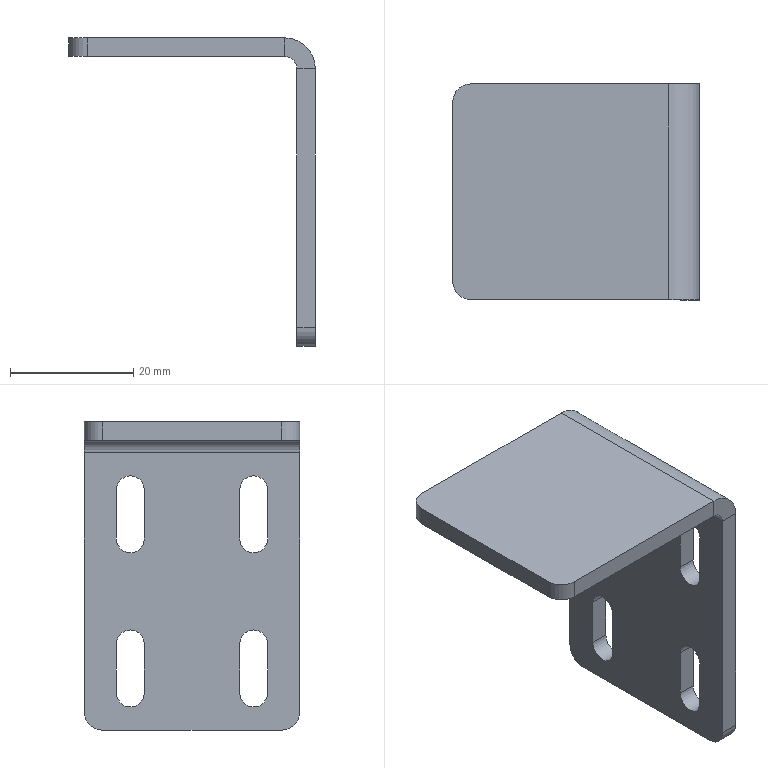Part | SolidWorks | features EdgeFlange 3, RefAxis 3, Fillet 2, ICE 2, FlatPattern 1, SMBaseFlange 1, SheetMetal 1 | 1 solid | 38 faces | box 40 x 35 x 50 mm | volume 8331 mm3 | plane 20 | cylinder 18 | commonest cylinder face diameters 4.5 x12 6 x4 4 x1 10 x1
STEP:
#1=CARTESIAN_POINT('',(55.,-7.75,-36.));
#2=VERTEX_POINT('',#1);
#3=CARTESIAN_POINT('',(55.,-10.,-33.75));
#4=VERTEX_POINT('',#3);
#5=CARTESIAN_POINT('',(55.,-10.,-36.));
#6=DIRECTION('',(1.,0.,0.));
#7=DIRECTION('',(0.,0.,-1.));
#8=AXIS2_PLACEMENT_3D('',#5,#6,#7);
#9=CIRCLE('',#8,2.25);
#10=EDGE_CURVE('',#2,#4,#9,.T.);
#11=ORIENTED_EDGE('',*,*,#10,.T.);
#12=CARTESIAN_POINT('',(52.,-10.,-33.75));
#13=VERTEX_POINT('',#12);
#14=CARTESIAN_POINT('',(62.,-10.,-33.75));
#15=DIRECTION('',(-1.,0.,0.));
#16=VECTOR('',#15,1000.);
#17=LINE('',#14,#16);
#18=EDGE_CURVE('',#4,#13,#17,.T.);
#19=ORIENTED_EDGE('',*,*,#18,.T.);
#20=CARTESIAN_POINT('',(52.,-7.75,-36.));
#21=VERTEX_POINT('',#20);
#22=CARTESIAN_POINT('',(52.,-10.,-36.));
#23=DIRECTION('',(-1.,0.,0.));
#24=DIRECTION('',(0.,0.,-1.));
#25=AXIS2_PLACEMENT_3D('',#22,#23,#24);
#26=CIRCLE('',#25,2.25);
#27=EDGE_CURVE('',#13,#21,#26,.T.);
#28=ORIENTED_EDGE('',*,*,#27,.T.);
#29=CARTESIAN_POINT('',(62.,-7.75,-36.));
#30=DIRECTION('',(-1.,0.,0.));
#31=VECTOR('',#30,1000.);
#32=LINE('',#29,#31);
#33=EDGE_CURVE('',#2,#21,#32,.T.);
#34=ORIENTED_EDGE('',*,*,#33,.F.);
#35=EDGE_LOOP('',(#11,#19,#28,#34));
#36=FACE_OUTER_BOUND('',#35,.T.);
#37=CARTESIAN_POINT('',(62.,-10.,-36.));
#38=DIRECTION('',(-1.,0.,0.));
#39=DIRECTION('',(0.,0.,1.));
#40=AXIS2_PLACEMENT_3D('',#37,#38,#39);
#41=CYLINDRICAL_SURFACE('',#40,2.25);
#42=ADVANCED_FACE('',(#36),#41,.F.);
#43=CARTESIAN_POINT('',(55.,-7.75,-11.));
#44=VERTEX_POINT('',#43);
#45=CARTESIAN_POINT('',(55.,-10.,-8.75));
#46=VERTEX_POINT('',#45);
#47=CARTESIAN_POINT('',(55.,-10.,-11.));
#48=DIRECTION('',(1.,0.,0.));
#49=DIRECTION('',(0.,0.,-1.));
#50=AXIS2_PLACEMENT_3D('',#47,#48,#49);
#51=CIRCLE('',#50,2.25);
#52=EDGE_CURVE('',#44,#46,#51,.T.);
#53=ORIENTED_EDGE('',*,*,#52,.T.);
#54=CARTESIAN_POINT('',(52.,-10.,-8.75));
#55=VERTEX_POINT('',#54);
#56=CARTESIAN_POINT('',(62.,-10.,-8.75));
#57=DIRECTION('',(-1.,0.,0.));
#58=VECTOR('',#57,1000.);
#59=LINE('',#56,#58);
#60=EDGE_CURVE('',#46,#55,#59,.T.);
#61=ORIENTED_EDGE('',*,*,#60,.T.);
#62=CARTESIAN_POINT('',(52.,-7.75,-11.));
#63=VERTEX_POINT('',#62);
#64=CARTESIAN_POINT('',(52.,-10.,-11.));
#65=DIRECTION('',(-1.,0.,0.));
#66=DIRECTION('',(0.,0.,1.));
#67=AXIS2_PLACEMENT_3D('',#64,#65,#66);
#68=CIRCLE('',#67,2.25);
#69=EDGE_CURVE('',#55,#63,#68,.T.);
#70=ORIENTED_EDGE('',*,*,#69,.T.);
#71=CARTESIAN_POINT('',(62.,-7.75,-11.));
#72=DIRECTION('',(-1.,0.,0.));
#73=VECTOR('',#72,1000.);
#74=LINE('',#71,#73);
#75=EDGE_CURVE('',#44,#63,#74,.T.);
#76=ORIENTED_EDGE('',*,*,#75,.F.);
#77=EDGE_LOOP('',(#53,#61,#70,#76));
#78=FACE_OUTER_BOUND('',#77,.T.);
#79=CARTESIAN_POINT('',(62.,-10.,-11.));
#80=DIRECTION('',(-1.,0.,0.));
#81=DIRECTION('',(0.,0.,1.));
#82=AXIS2_PLACEMENT_3D('',#79,#80,#81);
#83=CYLINDRICAL_SURFACE('',#82,2.25);
#84=ADVANCED_FACE('',(#78),#83,.F.);
#85=CARTESIAN_POINT('',(55.,12.25,-11.));
#86=VERTEX_POINT('',#85);
#87=CARTESIAN_POINT('',(55.,10.,-8.75));
#88=VERTEX_POINT('',#87);
#89=CARTESIAN_POINT('',(55.,10.,-11.));
#90=DIRECTION('',(1.,0.,0.));
#91=DIRECTION('',(0.,0.,-1.));
#92=AXIS2_PLACEMENT_3D('',#89,#90,#91);
#93=CIRCLE('',#92,2.25);
#94=EDGE_CURVE('',#86,#88,#93,.T.);
#95=ORIENTED_EDGE('',*,*,#94,.T.);
#96=CARTESIAN_POINT('',(52.,10.,-8.75));
#97=VERTEX_POINT('',#96);
#98=CARTESIAN_POINT('',(62.,10.,-8.75));
#99=DIRECTION('',(-1.,0.,0.));
#100=VECTOR('',#99,1000.);
#101=LINE('',#98,#100);
#102=EDGE_CURVE('',#88,#97,#101,.T.);
#103=ORIENTED_EDGE('',*,*,#102,.T.);
#104=CARTESIAN_POINT('',(52.,12.25,-11.));
#105=VERTEX_POINT('',#104);
#106=CARTESIAN_POINT('',(52.,10.,-11.));
#107=DIRECTION('',(-1.,0.,0.));
#108=DIRECTION('',(0.,0.,-1.));
#109=AXIS2_PLACEMENT_3D('',#106,#107,#108);
#110=CIRCLE('',#109,2.25);
#111=EDGE_CURVE('',#97,#105,#110,.T.);
#112=ORIENTED_EDGE('',*,*,#111,.T.);
#113=CARTESIAN_POINT('',(62.,12.25,-11.));
#114=DIRECTION('',(-1.,0.,0.));
#115=VECTOR('',#114,1000.);
#116=LINE('',#113,#115);
#117=EDGE_CURVE('',#86,#105,#116,.T.);
#118=ORIENTED_EDGE('',*,*,#117,.F.);
#119=EDGE_LOOP('',(#95,#103,#112,#118));
#120=FACE_OUTER_BOUND('',#119,.T.);
#121=CARTESIAN_POINT('',(62.,10.,-11.));
#122=DIRECTION('',(-1.,0.,0.));
#123=DIRECTION('',(0.,0.,1.));
#124=AXIS2_PLACEMENT_3D('',#121,#122,#123);
#125=CYLINDRICAL_SURFACE('',#124,2.25);
#126=ADVANCED_FACE('',(#120),#125,.F.);
#127=CARTESIAN_POINT('',(55.,12.25,-36.));
#128=VERTEX_POINT('',#127);
#129=CARTESIAN_POINT('',(55.,10.,-33.75));
#130=VERTEX_POINT('',#129);
#131=CARTESIAN_POINT('',(55.,10.,-36.));
#132=DIRECTION('',(1.,0.,0.));
#133=DIRECTION('',(0.,0.,-1.));
#134=AXIS2_PLACEMENT_3D('',#131,#132,#133);
#135=CIRCLE('',#134,2.25);
#136=EDGE_CURVE('',#128,#130,#135,.T.);
#137=ORIENTED_EDGE('',*,*,#136,.T.);
#138=CARTESIAN_POINT('',(52.,10.,-33.75));
#139=VERTEX_POINT('',#138);
#140=CARTESIAN_POINT('',(62.,10.,-33.75));
#141=DIRECTION('',(-1.,0.,0.));
#142=VECTOR('',#141,1000.);
#143=LINE('',#140,#142);
#144=EDGE_CURVE('',#130,#139,#143,.T.);
#145=ORIENTED_EDGE('',*,*,#144,.T.);
#146=CARTESIAN_POINT('',(52.,12.25,-36.));
#147=VERTEX_POINT('',#146);
#148=CARTESIAN_POINT('',(52.,10.,-36.));
#149=DIRECTION('',(-1.,0.,0.));
#150=DIRECTION('',(0.,0.,1.));
#151=AXIS2_PLACEMENT_3D('',#148,#149,#150);
#152=CIRCLE('',#151,2.25);
#153=EDGE_CURVE('',#139,#147,#152,.T.);
#154=ORIENTED_EDGE('',*,*,#153,.T.);
#155=CARTESIAN_POINT('',(62.,12.25,-36.));
#156=DIRECTION('',(-1.,0.,0.));
#157=VECTOR('',#156,1000.);
#158=LINE('',#155,#157);
#159=EDGE_CURVE('',#128,#147,#158,.T.);
#160=ORIENTED_EDGE('',*,*,#159,.F.);
#161=EDGE_LOOP('',(#137,#145,#154,#160));
#162=FACE_OUTER_BOUND('',#161,.T.);
#163=CARTESIAN_POINT('',(62.,10.,-36.));
#164=DIRECTION('',(-1.,0.,0.));
#165=DIRECTION('',(0.,0.,1.));
#166=AXIS2_PLACEMENT_3D('',#163,#164,#165);
#167=CYLINDRICAL_SURFACE('',#166,2.25);
#168=ADVANCED_FACE('',(#162),#167,.F.);
#169=CARTESIAN_POINT('',(18.,-17.5,0.));
#170=VERTEX_POINT('',#169);
#171=CARTESIAN_POINT('',(50.,-17.5,0.));
#172=VERTEX_POINT('',#171);
#173=CARTESIAN_POINT('',(-55.,-17.5,0.));
#174=DIRECTION('',(1.,0.,0.));
#175=VECTOR('',#174,1000.);
#176=LINE('',#173,#175);
#177=EDGE_CURVE('',#170,#172,#176,.T.);
#178=ORIENTED_EDGE('',*,*,#177,.F.);
#179=CARTESIAN_POINT('',(18.,-17.5,-3.));
#180=VERTEX_POINT('',#179);
#181=CARTESIAN_POINT('',(18.,-17.5,-3.));
#182=DIRECTION('',(0.,0.,-1.));
#183=VECTOR('',#182,1000.);
#184=LINE('',#181,#183);
#185=EDGE_CURVE('',#170,#180,#184,.T.);
#186=ORIENTED_EDGE('',*,*,#185,.T.);
#187=CARTESIAN_POINT('',(50.,-17.5,-3.));
#188=VERTEX_POINT('',#187);
#189=CARTESIAN_POINT('',(-55.,-17.5,-3.));
#190=DIRECTION('',(1.,0.,0.));
#191=VECTOR('',#190,1000.);
#192=LINE('',#189,#191);
#193=EDGE_CURVE('',#180,#188,#192,.T.);
#194=ORIENTED_EDGE('',*,*,#193,.T.);
#195=CARTESIAN_POINT('',(50.,-17.5,-3.));
#196=DIRECTION('',(0.,0.,1.));
#197=VECTOR('',#196,1000.);
#198=LINE('',#195,#197);
#199=EDGE_CURVE('',#188,#172,#198,.T.);
#200=ORIENTED_EDGE('',*,*,#199,.T.);
#201=EDGE_LOOP('',(#178,#186,#194,#200));
#202=FACE_OUTER_BOUND('',#201,.T.);
#203=CARTESIAN_POINT('',(-55.,-17.5,-3.));
#204=DIRECTION('',(0.,-1.,0.));
#205=DIRECTION('',(0.,0.,-1.));
#206=AXIS2_PLACEMENT_3D('',#203,#204,#205);
#207=PLANE('',#206);
#208=ADVANCED_FACE('',(#202),#207,.T.);
#209=ORIENTED_EDGE('',*,*,#193,.F.);
#210=CARTESIAN_POINT('',(15.,-14.5,-3.));
#211=VERTEX_POINT('',#210);
#212=CARTESIAN_POINT('',(18.,-14.5,-3.));
#213=DIRECTION('',(0.,0.,-1.));
#214=DIRECTION('',(-1.,0.,0.));
#215=AXIS2_PLACEMENT_3D('',#212,#213,#214);
#216=CIRCLE('',#215,3.);
#217=EDGE_CURVE('',#180,#211,#216,.T.);
#218=ORIENTED_EDGE('',*,*,#217,.T.);
#219=CARTESIAN_POINT('',(15.,14.5,-3.));
#220=VERTEX_POINT('',#219);
#221=CARTESIAN_POINT('',(15.,-17.5,-3.));
#222=DIRECTION('',(0.,1.,0.));
#223=VECTOR('',#222,1000.);
#224=LINE('',#221,#223);
#225=EDGE_CURVE('',#211,#220,#224,.T.);
#226=ORIENTED_EDGE('',*,*,#225,.T.);
#227=CARTESIAN_POINT('',(18.,17.5,-3.));
#228=VERTEX_POINT('',#227);
#229=CARTESIAN_POINT('',(18.,14.5,-3.));
#230=DIRECTION('',(0.,0.,-1.));
#231=DIRECTION('',(-1.,0.,0.));
#232=AXIS2_PLACEMENT_3D('',#229,#230,#231);
#233=CIRCLE('',#232,3.);
#234=EDGE_CURVE('',#220,#228,#233,.T.);
#235=ORIENTED_EDGE('',*,*,#234,.T.);
#236=CARTESIAN_POINT('',(50.,17.5,-3.));
#237=VERTEX_POINT('',#236);
#238=CARTESIAN_POINT('',(-55.,17.5,-3.));
#239=DIRECTION('',(-1.,0.,0.));
#240=VECTOR('',#239,1000.);
#241=LINE('',#238,#240);
#242=EDGE_CURVE('',#237,#228,#241,.T.);
#243=ORIENTED_EDGE('',*,*,#242,.F.);
#244=CARTESIAN_POINT('',(50.,-17.5,-3.));
#245=DIRECTION('',(0.,1.,0.));
#246=VECTOR('',#245,1000.);
#247=LINE('',#244,#246);
#248=EDGE_CURVE('',#188,#237,#247,.T.);
#249=ORIENTED_EDGE('',*,*,#248,.F.);
#250=EDGE_LOOP('',(#209,#218,#226,#235,#243,#249));
#251=FACE_OUTER_BOUND('',#250,.T.);
#252=CARTESIAN_POINT('',(0.,0.,-3.));
#253=DIRECTION('',(0.,0.,-1.));
#254=DIRECTION('',(-1.,0.,0.));
#255=AXIS2_PLACEMENT_3D('',#252,#253,#254);
#256=PLANE('',#255);
#257=ADVANCED_FACE('',(#251),#256,.T.);
#258=CARTESIAN_POINT('',(15.,14.5,0.));
#259=VERTEX_POINT('',#258);
#260=CARTESIAN_POINT('',(15.,-14.5,0.));
#261=VERTEX_POINT('',#260);
#262=CARTESIAN_POINT('',(15.,0.,0.));
#263=DIRECTION('',(0.,-1.,0.));
#264=VECTOR('',#263,1000.);
#265=LINE('',#262,#264);
#266=EDGE_CURVE('',#259,#261,#265,.T.);
#267=ORIENTED_EDGE('',*,*,#266,.T.);
#268=CARTESIAN_POINT('',(18.,-14.5,0.));
#269=DIRECTION('',(0.,0.,1.));
#270=DIRECTION('',(-1.,0.,0.));
#271=AXIS2_PLACEMENT_3D('',#268,#269,#270);
#272=CIRCLE('',#271,3.);
#273=EDGE_CURVE('',#261,#170,#272,.T.);
#274=ORIENTED_EDGE('',*,*,#273,.T.);
#275=ORIENTED_EDGE('',*,*,#177,.T.);
#276=CARTESIAN_POINT('',(50.,17.5,0.));
#277=VERTEX_POINT('',#276);
#278=CARTESIAN_POINT('',(50.,-17.5,0.));
#279=DIRECTION('',(0.,1.,0.));
#280=VECTOR('',#279,1000.);
#281=LINE('',#278,#280);
#282=EDGE_CURVE('',#172,#277,#281,.T.);
#283=ORIENTED_EDGE('',*,*,#282,.T.);
#284=CARTESIAN_POINT('',(18.,17.5,0.));
#285=VERTEX_POINT('',#284);
#286=CARTESIAN_POINT('',(-55.,17.5,0.));
#287=DIRECTION('',(-1.,0.,0.));
#288=VECTOR('',#287,1000.);
#289=LINE('',#286,#288);
#290=EDGE_CURVE('',#277,#285,#289,.T.);
#291=ORIENTED_EDGE('',*,*,#290,.T.);
#292=CARTESIAN_POINT('',(18.,14.5,0.));
#293=DIRECTION('',(0.,0.,1.));
#294=DIRECTION('',(-1.,0.,0.));
#295=AXIS2_PLACEMENT_3D('',#292,#293,#294);
#296=CIRCLE('',#295,3.);
#297=EDGE_CURVE('',#285,#259,#296,.T.);
#298=ORIENTED_EDGE('',*,*,#297,.T.);
#299=EDGE_LOOP('',(#267,#274,#275,#283,#291,#298));
#300=FACE_OUTER_BOUND('',#299,.T.);
#301=CARTESIAN_POINT('',(0.,0.,0.));
#302=DIRECTION('',(0.,0.,-1.));
#303=DIRECTION('',(-1.,0.,0.));
#304=AXIS2_PLACEMENT_3D('',#301,#302,#303);
#305=PLANE('',#304);
#306=ADVANCED_FACE('',(#300),#305,.F.);
#307=ORIENTED_EDGE('',*,*,#242,.T.);
#308=CARTESIAN_POINT('',(18.,17.5,0.));
#309=DIRECTION('',(0.,0.,1.));
#310=VECTOR('',#309,1000.);
#311=LINE('',#308,#310);
#312=EDGE_CURVE('',#228,#285,#311,.T.);
#313=ORIENTED_EDGE('',*,*,#312,.T.);
#314=ORIENTED_EDGE('',*,*,#290,.F.);
#315=CARTESIAN_POINT('',(50.,17.5,-3.));
#316=DIRECTION('',(0.,0.,1.));
#317=VECTOR('',#316,1000.);
#318=LINE('',#315,#317);
#319=EDGE_CURVE('',#237,#277,#318,.T.);
#320=ORIENTED_EDGE('',*,*,#319,.F.);
#321=EDGE_LOOP('',(#307,#313,#314,#320));
#322=FACE_OUTER_BOUND('',#321,.T.);
#323=CARTESIAN_POINT('',(-55.,17.5,-3.));
#324=DIRECTION('',(0.,1.,0.));
#325=DIRECTION('',(0.,0.,1.));
#326=AXIS2_PLACEMENT_3D('',#323,#324,#325);
#327=PLANE('',#326);
#328=ADVANCED_FACE('',(#322),#327,.T.);
#329=CARTESIAN_POINT('',(52.,17.5,-5.));
#330=VERTEX_POINT('',#329);
#331=CARTESIAN_POINT('',(55.,17.5,-5.));
#332=VERTEX_POINT('',#331);
#333=CARTESIAN_POINT('',(55.,17.5,-5.));
#334=DIRECTION('',(1.,0.,0.));
#335=VECTOR('',#334,1000.);
#336=LINE('',#333,#335);
#337=EDGE_CURVE('',#330,#332,#336,.T.);
#338=ORIENTED_EDGE('',*,*,#337,.F.);
#339=CARTESIAN_POINT('',(50.,17.5,-5.));
#340=DIRECTION('',(0.,1.,0.));
#341=DIRECTION('',(0.,0.,-1.));
#342=AXIS2_PLACEMENT_3D('',#339,#340,#341);
#343=CIRCLE('',#342,2.);
#344=EDGE_CURVE('',#237,#330,#343,.T.);
#345=ORIENTED_EDGE('',*,*,#344,.F.);
#346=ORIENTED_EDGE('',*,*,#319,.T.);
#347=CARTESIAN_POINT('',(50.,17.5,-5.));
#348=DIRECTION('',(0.,1.,0.));
#349=DIRECTION('',(0.,0.,-1.));
#350=AXIS2_PLACEMENT_3D('',#347,#348,#349);
#351=CIRCLE('',#350,5.);
#352=EDGE_CURVE('',#277,#332,#351,.T.);
#353=ORIENTED_EDGE('',*,*,#352,.T.);
#354=EDGE_LOOP('',(#338,#345,#346,#353));
#355=FACE_OUTER_BOUND('',#354,.T.);
#356=CARTESIAN_POINT('',(50.,17.5,-5.));
#357=DIRECTION('',(0.,1.,0.));
#358=DIRECTION('',(0.,0.,1.));
#359=AXIS2_PLACEMENT_3D('',#356,#357,#358);
#360=PLANE('',#359);
#361=ADVANCED_FACE('',(#355),#360,.T.);
#362=CARTESIAN_POINT('',(52.,-17.5,-5.));
#363=VERTEX_POINT('',#362);
#364=CARTESIAN_POINT('',(50.,-17.5,-5.));
#365=DIRECTION('',(0.,-1.,0.));
#366=DIRECTION('',(0.,0.,-1.));
#367=AXIS2_PLACEMENT_3D('',#364,#365,#366);
#368=CIRCLE('',#367,2.);
#369=EDGE_CURVE('',#363,#188,#368,.T.);
#370=ORIENTED_EDGE('',*,*,#369,.F.);
#371=CARTESIAN_POINT('',(55.,-17.5,-5.));
#372=VERTEX_POINT('',#371);
#373=CARTESIAN_POINT('',(52.,-17.5,-5.));
#374=DIRECTION('',(1.,0.,0.));
#375=VECTOR('',#374,1000.);
#376=LINE('',#373,#375);
#377=EDGE_CURVE('',#363,#372,#376,.T.);
#378=ORIENTED_EDGE('',*,*,#377,.T.);
#379=CARTESIAN_POINT('',(50.,-17.5,-5.));
#380=DIRECTION('',(0.,-1.,0.));
#381=DIRECTION('',(0.,0.,-1.));
#382=AXIS2_PLACEMENT_3D('',#379,#380,#381);
#383=CIRCLE('',#382,5.);
#384=EDGE_CURVE('',#372,#172,#383,.T.);
#385=ORIENTED_EDGE('',*,*,#384,.T.);
#386=ORIENTED_EDGE('',*,*,#199,.F.);
#387=EDGE_LOOP('',(#370,#378,#385,#386));
#388=FACE_OUTER_BOUND('',#387,.T.);
#389=CARTESIAN_POINT('',(50.,-17.5,-5.));
#390=DIRECTION('',(0.,1.,0.));
#391=DIRECTION('',(0.,0.,1.));
#392=AXIS2_PLACEMENT_3D('',#389,#390,#391);
#393=PLANE('',#392);
#394=ADVANCED_FACE('',(#388),#393,.F.);
#395=ORIENTED_EDGE('',*,*,#282,.F.);
#396=ORIENTED_EDGE('',*,*,#384,.F.);
#397=CARTESIAN_POINT('',(55.,0.,-5.));
#398=DIRECTION('',(0.,-1.,0.));
#399=VECTOR('',#398,1000.);
#400=LINE('',#397,#399);
#401=EDGE_CURVE('',#332,#372,#400,.T.);
#402=ORIENTED_EDGE('',*,*,#401,.F.);
#403=ORIENTED_EDGE('',*,*,#352,.F.);
#404=EDGE_LOOP('',(#395,#396,#402,#403));
#405=FACE_OUTER_BOUND('',#404,.T.);
#406=CARTESIAN_POINT('',(50.,-17.5,-5.));
#407=DIRECTION('',(0.,-1.,0.));
#408=DIRECTION('',(1.,0.,0.));
#409=AXIS2_PLACEMENT_3D('',#406,#407,#408);
#410=CYLINDRICAL_SURFACE('',#409,5.);
#411=ADVANCED_FACE('',(#405),#410,.T.);
#412=ORIENTED_EDGE('',*,*,#248,.T.);
#413=ORIENTED_EDGE('',*,*,#344,.T.);
#414=CARTESIAN_POINT('',(52.,17.5,-5.));
#415=DIRECTION('',(0.,-1.,0.));
#416=VECTOR('',#415,1000.);
#417=LINE('',#414,#416);
#418=EDGE_CURVE('',#330,#363,#417,.T.);
#419=ORIENTED_EDGE('',*,*,#418,.T.);
#420=ORIENTED_EDGE('',*,*,#369,.T.);
#421=EDGE_LOOP('',(#412,#413,#419,#420));
#422=FACE_OUTER_BOUND('',#421,.T.);
#423=CARTESIAN_POINT('',(50.,-17.5,-5.));
#424=DIRECTION('',(0.,-1.,0.));
#425=DIRECTION('',(1.,0.,0.));
#426=AXIS2_PLACEMENT_3D('',#423,#424,#425);
#427=CYLINDRICAL_SURFACE('',#426,2.);
#428=ADVANCED_FACE('',(#422),#427,.F.);
#429=CARTESIAN_POINT('',(52.,-17.5,-47.));
#430=VERTEX_POINT('',#429);
#431=CARTESIAN_POINT('',(52.,-17.5,0.));
#432=DIRECTION('',(0.,0.,1.));
#433=VECTOR('',#432,1000.);
#434=LINE('',#431,#433);
#435=EDGE_CURVE('',#430,#363,#434,.T.);
#436=ORIENTED_EDGE('',*,*,#435,.F.);
#437=CARTESIAN_POINT('',(55.,-17.5,-47.));
#438=VERTEX_POINT('',#437);
#439=CARTESIAN_POINT('',(55.,-17.5,-47.));
#440=DIRECTION('',(1.,0.,0.));
#441=VECTOR('',#440,1000.);
#442=LINE('',#439,#441);
#443=EDGE_CURVE('',#430,#438,#442,.T.);
#444=ORIENTED_EDGE('',*,*,#443,.T.);
#445=CARTESIAN_POINT('',(55.,-17.5,-3.));
#446=DIRECTION('',(0.,0.,1.));
#447=VECTOR('',#446,1000.);
#448=LINE('',#445,#447);
#449=EDGE_CURVE('',#438,#372,#448,.T.);
#450=ORIENTED_EDGE('',*,*,#449,.T.);
#451=ORIENTED_EDGE('',*,*,#377,.F.);
#452=EDGE_LOOP('',(#436,#444,#450,#451));
#453=FACE_OUTER_BOUND('',#452,.T.);
#454=CARTESIAN_POINT('',(55.,-17.5,-3.));
#455=DIRECTION('',(0.,-1.,0.));
#456=DIRECTION('',(0.,0.,-1.));
#457=AXIS2_PLACEMENT_3D('',#454,#455,#456);
#458=PLANE('',#457);
#459=ADVANCED_FACE('',(#453),#458,.T.);
#460=CARTESIAN_POINT('',(55.,17.5,-47.));
#461=VERTEX_POINT('',#460);
#462=CARTESIAN_POINT('',(55.,17.5,-50.));
#463=DIRECTION('',(0.,0.,-1.));
#464=VECTOR('',#463,1000.);
#465=LINE('',#462,#464);
#466=EDGE_CURVE('',#332,#461,#465,.T.);
#467=ORIENTED_EDGE('',*,*,#466,.T.);
#468=CARTESIAN_POINT('',(52.,17.5,-47.));
#469=VERTEX_POINT('',#468);
#470=CARTESIAN_POINT('',(55.,17.5,-47.));
#471=DIRECTION('',(-1.,0.,0.));
#472=VECTOR('',#471,1000.);
#473=LINE('',#470,#472);
#474=EDGE_CURVE('',#461,#469,#473,.T.);
#475=ORIENTED_EDGE('',*,*,#474,.T.);
#476=CARTESIAN_POINT('',(52.,17.5,0.));
#477=DIRECTION('',(0.,0.,-1.));
#478=VECTOR('',#477,1000.);
#479=LINE('',#476,#478);
#480=EDGE_CURVE('',#330,#469,#479,.T.);
#481=ORIENTED_EDGE('',*,*,#480,.F.);
#482=ORIENTED_EDGE('',*,*,#337,.T.);
#483=EDGE_LOOP('',(#467,#475,#481,#482));
#484=FACE_OUTER_BOUND('',#483,.T.);
#485=CARTESIAN_POINT('',(55.,17.5,-50.));
#486=DIRECTION('',(0.,1.,0.));
#487=DIRECTION('',(0.,0.,1.));
#488=AXIS2_PLACEMENT_3D('',#485,#486,#487);
#489=PLANE('',#488);
#490=ADVANCED_FACE('',(#484),#489,.T.);
#491=ORIENTED_EDGE('',*,*,#10,.F.);
#492=CARTESIAN_POINT('',(55.,-7.75,-44.));
#493=VERTEX_POINT('',#492);
#494=CARTESIAN_POINT('',(55.,-7.75,0.));
#495=DIRECTION('',(0.,0.,1.));
#496=VECTOR('',#495,1000.);
#497=LINE('',#494,#496);
#498=EDGE_CURVE('',#493,#2,#497,.T.);
#499=ORIENTED_EDGE('',*,*,#498,.F.);
#500=CARTESIAN_POINT('',(55.,-12.25,-44.));
#501=VERTEX_POINT('',#500);
#502=CARTESIAN_POINT('',(55.,-10.,-44.));
#503=DIRECTION('',(1.,0.,0.));
#504=DIRECTION('',(0.,0.,-1.));
#505=AXIS2_PLACEMENT_3D('',#502,#503,#504);
#506=CIRCLE('',#505,2.25);
#507=EDGE_CURVE('',#501,#493,#506,.T.);
#508=ORIENTED_EDGE('',*,*,#507,.F.);
#509=CARTESIAN_POINT('',(55.,-12.25,-36.));
#510=VERTEX_POINT('',#509);
#511=CARTESIAN_POINT('',(55.,-12.25,0.));
#512=DIRECTION('',(0.,0.,-1.));
#513=VECTOR('',#512,1000.);
#514=LINE('',#511,#513);
#515=EDGE_CURVE('',#510,#501,#514,.T.);
#516=ORIENTED_EDGE('',*,*,#515,.F.);
#517=CARTESIAN_POINT('',(55.,-10.,-36.));
#518=DIRECTION('',(1.,0.,0.));
#519=DIRECTION('',(0.,0.,-1.));
#520=AXIS2_PLACEMENT_3D('',#517,#518,#519);
#521=CIRCLE('',#520,2.25);
#522=EDGE_CURVE('',#4,#510,#521,.T.);
#523=ORIENTED_EDGE('',*,*,#522,.F.);
#524=EDGE_LOOP('',(#491,#499,#508,#516,#523));
#525=FACE_BOUND('',#524,.T.);
#526=CARTESIAN_POINT('',(55.,-12.25,-19.));
#527=VERTEX_POINT('',#526);
#528=CARTESIAN_POINT('',(55.,-7.75,-19.));
#529=VERTEX_POINT('',#528);
#530=CARTESIAN_POINT('',(55.,-10.,-19.));
#531=DIRECTION('',(1.,0.,0.));
#532=DIRECTION('',(0.,0.,-1.));
#533=AXIS2_PLACEMENT_3D('',#530,#531,#532);
#534=CIRCLE('',#533,2.25);
#535=EDGE_CURVE('',#527,#529,#534,.T.);
#536=ORIENTED_EDGE('',*,*,#535,.F.);
#537=CARTESIAN_POINT('',(55.,-12.25,-11.));
#538=VERTEX_POINT('',#537);
#539=CARTESIAN_POINT('',(55.,-12.25,0.));
#540=DIRECTION('',(0.,0.,-1.));
#541=VECTOR('',#540,1000.);
#542=LINE('',#539,#541);
#543=EDGE_CURVE('',#538,#527,#542,.T.);
#544=ORIENTED_EDGE('',*,*,#543,.F.);
#545=CARTESIAN_POINT('',(55.,-10.,-11.));
#546=DIRECTION('',(1.,0.,0.));
#547=DIRECTION('',(0.,0.,-1.));
#548=AXIS2_PLACEMENT_3D('',#545,#546,#547);
#549=CIRCLE('',#548,2.25);
#550=EDGE_CURVE('',#46,#538,#549,.T.);
#551=ORIENTED_EDGE('',*,*,#550,.F.);
#552=ORIENTED_EDGE('',*,*,#52,.F.);
#553=CARTESIAN_POINT('',(55.,-7.75,0.));
#554=DIRECTION('',(0.,0.,1.));
#555=VECTOR('',#554,1000.);
#556=LINE('',#553,#555);
#557=EDGE_CURVE('',#529,#44,#556,.T.);
#558=ORIENTED_EDGE('',*,*,#557,.F.);
#559=EDGE_LOOP('',(#536,#544,#551,#552,#558));
#560=FACE_BOUND('',#559,.T.);
#561=CARTESIAN_POINT('',(55.,7.75,-19.));
#562=VERTEX_POINT('',#561);
#563=CARTESIAN_POINT('',(55.,12.25,-19.));
#564=VERTEX_POINT('',#563);
#565=CARTESIAN_POINT('',(55.,10.,-19.));
#566=DIRECTION('',(1.,0.,0.));
#567=DIRECTION('',(0.,0.,-1.));
#568=AXIS2_PLACEMENT_3D('',#565,#566,#567);
#569=CIRCLE('',#568,2.25);
#570=EDGE_CURVE('',#562,#564,#569,.T.);
#571=ORIENTED_EDGE('',*,*,#570,.F.);
#572=CARTESIAN_POINT('',(55.,7.75,-11.));
#573=VERTEX_POINT('',#572);
#574=CARTESIAN_POINT('',(55.,7.75,0.));
#575=DIRECTION('',(0.,0.,-1.));
#576=VECTOR('',#575,1000.);
#577=LINE('',#574,#576);
#578=EDGE_CURVE('',#573,#562,#577,.T.);
#579=ORIENTED_EDGE('',*,*,#578,.F.);
#580=CARTESIAN_POINT('',(55.,10.,-11.));
#581=DIRECTION('',(1.,0.,0.));
#582=DIRECTION('',(0.,0.,-1.));
#583=AXIS2_PLACEMENT_3D('',#580,#581,#582);
#584=CIRCLE('',#583,2.25);
#585=EDGE_CURVE('',#88,#573,#584,.T.);
#586=ORIENTED_EDGE('',*,*,#585,.F.);
#587=ORIENTED_EDGE('',*,*,#94,.F.);
#588=CARTESIAN_POINT('',(55.,12.25,0.));
#589=DIRECTION('',(0.,0.,1.));
#590=VECTOR('',#589,1000.);
#591=LINE('',#588,#590);
#592=EDGE_CURVE('',#564,#86,#591,.T.);
#593=ORIENTED_EDGE('',*,*,#592,.F.);
#594=EDGE_LOOP('',(#571,#579,#586,#587,#593));
#595=FACE_BOUND('',#594,.T.);
#596=ORIENTED_EDGE('',*,*,#136,.F.);
#597=CARTESIAN_POINT('',(55.,12.25,-44.));
#598=VERTEX_POINT('',#597);
#599=CARTESIAN_POINT('',(55.,12.25,0.));
#600=DIRECTION('',(0.,0.,1.));
#601=VECTOR('',#600,1000.);
#602=LINE('',#599,#601);
#603=EDGE_CURVE('',#598,#128,#602,.T.);
#604=ORIENTED_EDGE('',*,*,#603,.F.);
#605=CARTESIAN_POINT('',(55.,7.75,-44.));
#606=VERTEX_POINT('',#605);
#607=CARTESIAN_POINT('',(55.,10.,-44.));
#608=DIRECTION('',(1.,0.,0.));
#609=DIRECTION('',(0.,0.,-1.));
#610=AXIS2_PLACEMENT_3D('',#607,#608,#609);
#611=CIRCLE('',#610,2.25);
#612=EDGE_CURVE('',#606,#598,#611,.T.);
#613=ORIENTED_EDGE('',*,*,#612,.F.);
#614=CARTESIAN_POINT('',(55.,7.75,-36.));
#615=VERTEX_POINT('',#614);
#616=CARTESIAN_POINT('',(55.,7.75,0.));
#617=DIRECTION('',(0.,0.,-1.));
#618=VECTOR('',#617,1000.);
#619=LINE('',#616,#618);
#620=EDGE_CURVE('',#615,#606,#619,.T.);
#621=ORIENTED_EDGE('',*,*,#620,.F.);
#622=CARTESIAN_POINT('',(55.,10.,-36.));
#623=DIRECTION('',(1.,0.,0.));
#624=DIRECTION('',(0.,0.,-1.));
#625=AXIS2_PLACEMENT_3D('',#622,#623,#624);
#626=CIRCLE('',#625,2.25);
#627=EDGE_CURVE('',#130,#615,#626,.T.);
#628=ORIENTED_EDGE('',*,*,#627,.F.);
#629=EDGE_LOOP('',(#596,#604,#613,#621,#628));
#630=FACE_BOUND('',#629,.T.);
#631=ORIENTED_EDGE('',*,*,#449,.F.);
#632=CARTESIAN_POINT('',(55.,-14.5,-50.));
#633=VERTEX_POINT('',#632);
#634=CARTESIAN_POINT('',(55.,-14.5,-47.));
#635=DIRECTION('',(1.,0.,0.));
#636=DIRECTION('',(0.,0.,-1.));
#637=AXIS2_PLACEMENT_3D('',#634,#635,#636);
#638=CIRCLE('',#637,3.);
#639=EDGE_CURVE('',#438,#633,#638,.T.);
#640=ORIENTED_EDGE('',*,*,#639,.T.);
#641=CARTESIAN_POINT('',(55.,14.5,-50.));
#642=VERTEX_POINT('',#641);
#643=CARTESIAN_POINT('',(55.,-17.5,-50.));
#644=DIRECTION('',(0.,-1.,0.));
#645=VECTOR('',#644,1000.);
#646=LINE('',#643,#645);
#647=EDGE_CURVE('',#642,#633,#646,.T.);
#648=ORIENTED_EDGE('',*,*,#647,.F.);
#649=CARTESIAN_POINT('',(55.,14.5,-47.));
#650=DIRECTION('',(1.,0.,0.));
#651=DIRECTION('',(0.,0.,-1.));
#652=AXIS2_PLACEMENT_3D('',#649,#650,#651);
#653=CIRCLE('',#652,3.);
#654=EDGE_CURVE('',#642,#461,#653,.T.);
#655=ORIENTED_EDGE('',*,*,#654,.T.);
#656=ORIENTED_EDGE('',*,*,#466,.F.);
#657=ORIENTED_EDGE('',*,*,#401,.T.);
#658=EDGE_LOOP('',(#631,#640,#648,#655,#656,#657));
#659=FACE_OUTER_BOUND('',#658,.T.);
#660=CARTESIAN_POINT('',(55.,0.,0.));
#661=DIRECTION('',(1.,0.,0.));
#662=DIRECTION('',(0.,0.,-1.));
#663=AXIS2_PLACEMENT_3D('',#660,#661,#662);
#664=PLANE('',#663);
#665=ADVANCED_FACE('',(#525,#560,#595,#630,#659),#664,.T.);
#666=CARTESIAN_POINT('',(52.,-7.75,-44.));
#667=VERTEX_POINT('',#666);
#668=CARTESIAN_POINT('',(52.,-7.75,-36.));
#669=DIRECTION('',(0.,0.,-1.));
#670=VECTOR('',#669,1000.);
#671=LINE('',#668,#670);
#672=EDGE_CURVE('',#21,#667,#671,.T.);
#673=ORIENTED_EDGE('',*,*,#672,.F.);
#674=ORIENTED_EDGE('',*,*,#27,.F.);
#675=CARTESIAN_POINT('',(52.,-12.25,-36.));
#676=VERTEX_POINT('',#675);
#677=CARTESIAN_POINT('',(52.,-10.,-36.));
#678=DIRECTION('',(-1.,0.,0.));
#679=DIRECTION('',(0.,0.,-1.));
#680=AXIS2_PLACEMENT_3D('',#677,#678,#679);
#681=CIRCLE('',#680,2.25);
#682=EDGE_CURVE('',#676,#13,#681,.T.);
#683=ORIENTED_EDGE('',*,*,#682,.F.);
#684=CARTESIAN_POINT('',(52.,-12.25,-44.));
#685=VERTEX_POINT('',#684);
#686=CARTESIAN_POINT('',(52.,-12.25,-36.));
#687=DIRECTION('',(0.,0.,1.));
#688=VECTOR('',#687,1000.);
#689=LINE('',#686,#688);
#690=EDGE_CURVE('',#685,#676,#689,.T.);
#691=ORIENTED_EDGE('',*,*,#690,.F.);
#692=CARTESIAN_POINT('',(52.,-10.,-44.));
#693=DIRECTION('',(-1.,0.,0.));
#694=DIRECTION('',(0.,0.,-1.));
#695=AXIS2_PLACEMENT_3D('',#692,#693,#694);
#696=CIRCLE('',#695,2.25);
#697=EDGE_CURVE('',#667,#685,#696,.T.);
#698=ORIENTED_EDGE('',*,*,#697,.F.);
#699=EDGE_LOOP('',(#673,#674,#683,#691,#698));
#700=FACE_BOUND('',#699,.T.);
#701=CARTESIAN_POINT('',(52.,-12.25,-19.));
#702=VERTEX_POINT('',#701);
#703=CARTESIAN_POINT('',(52.,-12.25,-11.));
#704=VERTEX_POINT('',#703);
#705=CARTESIAN_POINT('',(52.,-12.25,-19.));
#706=DIRECTION('',(0.,0.,1.));
#707=VECTOR('',#706,1000.);
#708=LINE('',#705,#707);
#709=EDGE_CURVE('',#702,#704,#708,.T.);
#710=ORIENTED_EDGE('',*,*,#709,.F.);
#711=CARTESIAN_POINT('',(52.,-7.75,-19.));
#712=VERTEX_POINT('',#711);
#713=CARTESIAN_POINT('',(52.,-10.,-19.));
#714=DIRECTION('',(-1.,0.,0.));
#715=DIRECTION('',(0.,0.,1.));
#716=AXIS2_PLACEMENT_3D('',#713,#714,#715);
#717=CIRCLE('',#716,2.25);
#718=EDGE_CURVE('',#712,#702,#717,.T.);
#719=ORIENTED_EDGE('',*,*,#718,.F.);
#720=CARTESIAN_POINT('',(52.,-7.75,-19.));
#721=DIRECTION('',(0.,0.,-1.));
#722=VECTOR('',#721,1000.);
#723=LINE('',#720,#722);
#724=EDGE_CURVE('',#63,#712,#723,.T.);
#725=ORIENTED_EDGE('',*,*,#724,.F.);
#726=ORIENTED_EDGE('',*,*,#69,.F.);
#727=CARTESIAN_POINT('',(52.,-10.,-11.));
#728=DIRECTION('',(-1.,0.,0.));
#729=DIRECTION('',(0.,0.,1.));
#730=AXIS2_PLACEMENT_3D('',#727,#728,#729);
#731=CIRCLE('',#730,2.25);
#732=EDGE_CURVE('',#704,#55,#731,.T.);
#733=ORIENTED_EDGE('',*,*,#732,.F.);
#734=EDGE_LOOP('',(#710,#719,#725,#726,#733));
#735=FACE_BOUND('',#734,.T.);
#736=CARTESIAN_POINT('',(52.,7.75,-19.));
#737=VERTEX_POINT('',#736);
#738=CARTESIAN_POINT('',(52.,7.75,-11.));
#739=VERTEX_POINT('',#738);
#740=CARTESIAN_POINT('',(52.,7.75,-19.));
#741=DIRECTION('',(0.,0.,1.));
#742=VECTOR('',#741,1000.);
#743=LINE('',#740,#742);
#744=EDGE_CURVE('',#737,#739,#743,.T.);
#745=ORIENTED_EDGE('',*,*,#744,.F.);
#746=CARTESIAN_POINT('',(52.,12.25,-19.));
#747=VERTEX_POINT('',#746);
#748=CARTESIAN_POINT('',(52.,10.,-19.));
#749=DIRECTION('',(-1.,0.,0.));
#750=DIRECTION('',(0.,0.,-1.));
#751=AXIS2_PLACEMENT_3D('',#748,#749,#750);
#752=CIRCLE('',#751,2.25);
#753=EDGE_CURVE('',#747,#737,#752,.T.);
#754=ORIENTED_EDGE('',*,*,#753,.F.);
#755=CARTESIAN_POINT('',(52.,12.25,-19.));
#756=DIRECTION('',(0.,0.,-1.));
#757=VECTOR('',#756,1000.);
#758=LINE('',#755,#757);
#759=EDGE_CURVE('',#105,#747,#758,.T.);
#760=ORIENTED_EDGE('',*,*,#759,.F.);
#761=ORIENTED_EDGE('',*,*,#111,.F.);
#762=CARTESIAN_POINT('',(52.,10.,-11.));
#763=DIRECTION('',(-1.,0.,0.));
#764=DIRECTION('',(0.,0.,-1.));
#765=AXIS2_PLACEMENT_3D('',#762,#763,#764);
#766=CIRCLE('',#765,2.25);
#767=EDGE_CURVE('',#739,#97,#766,.T.);
#768=ORIENTED_EDGE('',*,*,#767,.F.);
#769=EDGE_LOOP('',(#745,#754,#760,#761,#768));
#770=FACE_BOUND('',#769,.T.);
#771=CARTESIAN_POINT('',(52.,12.25,-44.));
#772=VERTEX_POINT('',#771);
#773=CARTESIAN_POINT('',(52.,12.25,-36.));
#774=DIRECTION('',(0.,0.,-1.));
#775=VECTOR('',#774,1000.);
#776=LINE('',#773,#775);
#777=EDGE_CURVE('',#147,#772,#776,.T.);
#778=ORIENTED_EDGE('',*,*,#777,.F.);
#779=ORIENTED_EDGE('',*,*,#153,.F.);
#780=CARTESIAN_POINT('',(52.,7.75,-36.));
#781=VERTEX_POINT('',#780);
#782=CARTESIAN_POINT('',(52.,10.,-36.));
#783=DIRECTION('',(-1.,0.,0.));
#784=DIRECTION('',(0.,0.,1.));
#785=AXIS2_PLACEMENT_3D('',#782,#783,#784);
#786=CIRCLE('',#785,2.25);
#787=EDGE_CURVE('',#781,#139,#786,.T.);
#788=ORIENTED_EDGE('',*,*,#787,.F.);
#789=CARTESIAN_POINT('',(52.,7.75,-44.));
#790=VERTEX_POINT('',#789);
#791=CARTESIAN_POINT('',(52.,7.75,-36.));
#792=DIRECTION('',(0.,0.,1.));
#793=VECTOR('',#792,1000.);
#794=LINE('',#791,#793);
#795=EDGE_CURVE('',#790,#781,#794,.T.);
#796=ORIENTED_EDGE('',*,*,#795,.F.);
#797=CARTESIAN_POINT('',(52.,10.,-44.));
#798=DIRECTION('',(-1.,0.,0.));
#799=DIRECTION('',(0.,0.,1.));
#800=AXIS2_PLACEMENT_3D('',#797,#798,#799);
#801=CIRCLE('',#800,2.25);
#802=EDGE_CURVE('',#772,#790,#801,.T.);
#803=ORIENTED_EDGE('',*,*,#802,.F.);
#804=EDGE_LOOP('',(#778,#779,#788,#796,#803));
#805=FACE_BOUND('',#804,.T.);
#806=CARTESIAN_POINT('',(52.,14.5,-50.));
#807=VERTEX_POINT('',#806);
#808=CARTESIAN_POINT('',(52.,-14.5,-50.));
#809=VERTEX_POINT('',#808);
#810=CARTESIAN_POINT('',(52.,0.,-50.));
#811=DIRECTION('',(0.,-1.,0.));
#812=VECTOR('',#811,1000.);
#813=LINE('',#810,#812);
#814=EDGE_CURVE('',#807,#809,#813,.T.);
#815=ORIENTED_EDGE('',*,*,#814,.T.);
#816=CARTESIAN_POINT('',(52.,-14.5,-47.));
#817=DIRECTION('',(-1.,0.,0.));
#818=DIRECTION('',(0.,0.,-1.));
#819=AXIS2_PLACEMENT_3D('',#816,#817,#818);
#820=CIRCLE('',#819,3.);
#821=EDGE_CURVE('',#809,#430,#820,.T.);
#822=ORIENTED_EDGE('',*,*,#821,.T.);
#823=ORIENTED_EDGE('',*,*,#435,.T.);
#824=ORIENTED_EDGE('',*,*,#418,.F.);
#825=ORIENTED_EDGE('',*,*,#480,.T.);
#826=CARTESIAN_POINT('',(52.,14.5,-47.));
#827=DIRECTION('',(-1.,0.,0.));
#828=DIRECTION('',(0.,0.,-1.));
#829=AXIS2_PLACEMENT_3D('',#826,#827,#828);
#830=CIRCLE('',#829,3.);
#831=EDGE_CURVE('',#469,#807,#830,.T.);
#832=ORIENTED_EDGE('',*,*,#831,.T.);
#833=EDGE_LOOP('',(#815,#822,#823,#824,#825,#832));
#834=FACE_OUTER_BOUND('',#833,.T.);
#835=CARTESIAN_POINT('',(52.,0.,0.));
#836=DIRECTION('',(1.,0.,0.));
#837=DIRECTION('',(0.,0.,-1.));
#838=AXIS2_PLACEMENT_3D('',#835,#836,#837);
#839=PLANE('',#838);
#840=ADVANCED_FACE('',(#700,#735,#770,#805,#834),#839,.F.);
#841=ORIENTED_EDGE('',*,*,#647,.T.);
#842=CARTESIAN_POINT('',(55.,-14.5,-50.));
#843=DIRECTION('',(-1.,0.,0.));
#844=VECTOR('',#843,1000.);
#845=LINE('',#842,#844);
#846=EDGE_CURVE('',#633,#809,#845,.T.);
#847=ORIENTED_EDGE('',*,*,#846,.T.);
#848=ORIENTED_EDGE('',*,*,#814,.F.);
#849=CARTESIAN_POINT('',(55.,14.5,-50.));
#850=DIRECTION('',(1.,0.,0.));
#851=VECTOR('',#850,1000.);
#852=LINE('',#849,#851);
#853=EDGE_CURVE('',#807,#642,#852,.T.);
#854=ORIENTED_EDGE('',*,*,#853,.T.);
#855=EDGE_LOOP('',(#841,#847,#848,#854));
#856=FACE_OUTER_BOUND('',#855,.T.);
#857=CARTESIAN_POINT('',(55.,-17.5,-50.));
#858=DIRECTION('',(0.,0.,-1.));
#859=DIRECTION('',(-1.,0.,0.));
#860=AXIS2_PLACEMENT_3D('',#857,#858,#859);
#861=PLANE('',#860);
#862=ADVANCED_FACE('',(#856),#861,.T.);
#863=ORIENTED_EDGE('',*,*,#639,.F.);
#864=ORIENTED_EDGE('',*,*,#443,.F.);
#865=ORIENTED_EDGE('',*,*,#821,.F.);
#866=ORIENTED_EDGE('',*,*,#846,.F.);
#867=EDGE_LOOP('',(#863,#864,#865,#866));
#868=FACE_OUTER_BOUND('',#867,.T.);
#869=CARTESIAN_POINT('',(55.,-14.5,-47.));
#870=DIRECTION('',(-1.,0.,0.));
#871=DIRECTION('',(0.,0.,1.));
#872=AXIS2_PLACEMENT_3D('',#869,#870,#871);
#873=CYLINDRICAL_SURFACE('',#872,3.);
#874=ADVANCED_FACE('',(#868),#873,.T.);
#875=ORIENTED_EDGE('',*,*,#654,.F.);
#876=ORIENTED_EDGE('',*,*,#853,.F.);
#877=ORIENTED_EDGE('',*,*,#831,.F.);
#878=ORIENTED_EDGE('',*,*,#474,.F.);
#879=EDGE_LOOP('',(#875,#876,#877,#878));
#880=FACE_OUTER_BOUND('',#879,.T.);
#881=CARTESIAN_POINT('',(55.,14.5,-47.));
#882=DIRECTION('',(-1.,0.,0.));
#883=DIRECTION('',(0.,0.,1.));
#884=AXIS2_PLACEMENT_3D('',#881,#882,#883);
#885=CYLINDRICAL_SURFACE('',#884,3.);
#886=ADVANCED_FACE('',(#880),#885,.T.);
#887=ORIENTED_EDGE('',*,*,#144,.F.);
#888=ORIENTED_EDGE('',*,*,#627,.T.);
#889=CARTESIAN_POINT('',(62.,7.75,-36.));
#890=DIRECTION('',(-1.,0.,0.));
#891=VECTOR('',#890,1000.);
#892=LINE('',#889,#891);
#893=EDGE_CURVE('',#615,#781,#892,.T.);
#894=ORIENTED_EDGE('',*,*,#893,.T.);
#895=ORIENTED_EDGE('',*,*,#787,.T.);
#896=EDGE_LOOP('',(#887,#888,#894,#895));
#897=FACE_OUTER_BOUND('',#896,.T.);
#898=CARTESIAN_POINT('',(62.,10.,-36.));
#899=DIRECTION('',(-1.,0.,0.));
#900=DIRECTION('',(0.,0.,1.));
#901=AXIS2_PLACEMENT_3D('',#898,#899,#900);
#902=CYLINDRICAL_SURFACE('',#901,2.25);
#903=ADVANCED_FACE('',(#897),#902,.F.);
#904=ORIENTED_EDGE('',*,*,#620,.T.);
#905=CARTESIAN_POINT('',(62.,7.75,-44.));
#906=DIRECTION('',(-1.,0.,0.));
#907=VECTOR('',#906,1000.);
#908=LINE('',#905,#907);
#909=EDGE_CURVE('',#606,#790,#908,.T.);
#910=ORIENTED_EDGE('',*,*,#909,.T.);
#911=ORIENTED_EDGE('',*,*,#795,.T.);
#912=ORIENTED_EDGE('',*,*,#893,.F.);
#913=EDGE_LOOP('',(#904,#910,#911,#912));
#914=FACE_OUTER_BOUND('',#913,.T.);
#915=CARTESIAN_POINT('',(62.,7.75,-36.));
#916=DIRECTION('',(0.,-1.,0.));
#917=DIRECTION('',(0.,0.,-1.));
#918=AXIS2_PLACEMENT_3D('',#915,#916,#917);
#919=PLANE('',#918);
#920=ADVANCED_FACE('',(#914),#919,.F.);
#921=ORIENTED_EDGE('',*,*,#612,.T.);
#922=CARTESIAN_POINT('',(62.,12.25,-44.));
#923=DIRECTION('',(-1.,0.,0.));
#924=VECTOR('',#923,1000.);
#925=LINE('',#922,#924);
#926=EDGE_CURVE('',#598,#772,#925,.T.);
#927=ORIENTED_EDGE('',*,*,#926,.T.);
#928=ORIENTED_EDGE('',*,*,#802,.T.);
#929=ORIENTED_EDGE('',*,*,#909,.F.);
#930=EDGE_LOOP('',(#921,#927,#928,#929));
#931=FACE_OUTER_BOUND('',#930,.T.);
#932=CARTESIAN_POINT('',(62.,10.,-44.));
#933=DIRECTION('',(-1.,0.,0.));
#934=DIRECTION('',(0.,0.,1.));
#935=AXIS2_PLACEMENT_3D('',#932,#933,#934);
#936=CYLINDRICAL_SURFACE('',#935,2.25);
#937=ADVANCED_FACE('',(#931),#936,.F.);
#938=ORIENTED_EDGE('',*,*,#603,.T.);
#939=ORIENTED_EDGE('',*,*,#159,.T.);
#940=ORIENTED_EDGE('',*,*,#777,.T.);
#941=ORIENTED_EDGE('',*,*,#926,.F.);
#942=EDGE_LOOP('',(#938,#939,#940,#941));
#943=FACE_OUTER_BOUND('',#942,.T.);
#944=CARTESIAN_POINT('',(62.,12.25,-36.));
#945=DIRECTION('',(0.,1.,0.));
#946=DIRECTION('',(0.,0.,1.));
#947=AXIS2_PLACEMENT_3D('',#944,#945,#946);
#948=PLANE('',#947);
#949=ADVANCED_FACE('',(#943),#948,.F.);
#950=ORIENTED_EDGE('',*,*,#570,.T.);
#951=CARTESIAN_POINT('',(62.,12.25,-19.));
#952=DIRECTION('',(-1.,0.,0.));
#953=VECTOR('',#952,1000.);
#954=LINE('',#951,#953);
#955=EDGE_CURVE('',#564,#747,#954,.T.);
#956=ORIENTED_EDGE('',*,*,#955,.T.);
#957=ORIENTED_EDGE('',*,*,#753,.T.);
#958=CARTESIAN_POINT('',(62.,7.75,-19.));
#959=DIRECTION('',(-1.,0.,0.));
#960=VECTOR('',#959,1000.);
#961=LINE('',#958,#960);
#962=EDGE_CURVE('',#562,#737,#961,.T.);
#963=ORIENTED_EDGE('',*,*,#962,.F.);
#964=EDGE_LOOP('',(#950,#956,#957,#963));
#965=FACE_OUTER_BOUND('',#964,.T.);
#966=CARTESIAN_POINT('',(62.,10.,-19.));
#967=DIRECTION('',(-1.,0.,0.));
#968=DIRECTION('',(0.,0.,1.));
#969=AXIS2_PLACEMENT_3D('',#966,#967,#968);
#970=CYLINDRICAL_SURFACE('',#969,2.25);
#971=ADVANCED_FACE('',(#965),#970,.F.);
#972=ORIENTED_EDGE('',*,*,#592,.T.);
#973=ORIENTED_EDGE('',*,*,#117,.T.);
#974=ORIENTED_EDGE('',*,*,#759,.T.);
#975=ORIENTED_EDGE('',*,*,#955,.F.);
#976=EDGE_LOOP('',(#972,#973,#974,#975));
#977=FACE_OUTER_BOUND('',#976,.T.);
#978=CARTESIAN_POINT('',(62.,12.25,-19.));
#979=DIRECTION('',(0.,1.,0.));
#980=DIRECTION('',(0.,0.,1.));
#981=AXIS2_PLACEMENT_3D('',#978,#979,#980);
#982=PLANE('',#981);
#983=ADVANCED_FACE('',(#977),#982,.F.);
#984=ORIENTED_EDGE('',*,*,#102,.F.);
#985=ORIENTED_EDGE('',*,*,#585,.T.);
#986=CARTESIAN_POINT('',(62.,7.75,-11.));
#987=DIRECTION('',(-1.,0.,0.));
#988=VECTOR('',#987,1000.);
#989=LINE('',#986,#988);
#990=EDGE_CURVE('',#573,#739,#989,.T.);
#991=ORIENTED_EDGE('',*,*,#990,.T.);
#992=ORIENTED_EDGE('',*,*,#767,.T.);
#993=EDGE_LOOP('',(#984,#985,#991,#992));
#994=FACE_OUTER_BOUND('',#993,.T.);
#995=CARTESIAN_POINT('',(62.,10.,-11.));
#996=DIRECTION('',(-1.,0.,0.));
#997=DIRECTION('',(0.,0.,1.));
#998=AXIS2_PLACEMENT_3D('',#995,#996,#997);
#999=CYLINDRICAL_SURFACE('',#998,2.25);
#1000=ADVANCED_FACE('',(#994),#999,.F.);
#1001=ORIENTED_EDGE('',*,*,#578,.T.);
#1002=ORIENTED_EDGE('',*,*,#962,.T.);
#1003=ORIENTED_EDGE('',*,*,#744,.T.);
#1004=ORIENTED_EDGE('',*,*,#990,.F.);
#1005=EDGE_LOOP('',(#1001,#1002,#1003,#1004));
#1006=FACE_OUTER_BOUND('',#1005,.T.);
#1007=CARTESIAN_POINT('',(62.,7.75,-19.));
#1008=DIRECTION('',(0.,-1.,0.));
#1009=DIRECTION('',(0.,0.,-1.));
#1010=AXIS2_PLACEMENT_3D('',#1007,#1008,#1009);
#1011=PLANE('',#1010);
#1012=ADVANCED_FACE('',(#1006),#1011,.F.);
#1013=ORIENTED_EDGE('',*,*,#535,.T.);
#1014=CARTESIAN_POINT('',(62.,-7.75,-19.));
#1015=DIRECTION('',(-1.,0.,0.));
#1016=VECTOR('',#1015,1000.);
#1017=LINE('',#1014,#1016);
#1018=EDGE_CURVE('',#529,#712,#1017,.T.);
#1019=ORIENTED_EDGE('',*,*,#1018,.T.);
#1020=ORIENTED_EDGE('',*,*,#718,.T.);
#1021=CARTESIAN_POINT('',(62.,-12.25,-19.));
#1022=DIRECTION('',(-1.,0.,0.));
#1023=VECTOR('',#1022,1000.);
#1024=LINE('',#1021,#1023);
#1025=EDGE_CURVE('',#527,#702,#1024,.T.);
#1026=ORIENTED_EDGE('',*,*,#1025,.F.);
#1027=EDGE_LOOP('',(#1013,#1019,#1020,#1026));
#1028=FACE_OUTER_BOUND('',#1027,.T.);
#1029=CARTESIAN_POINT('',(62.,-10.,-19.));
#1030=DIRECTION('',(-1.,0.,0.));
#1031=DIRECTION('',(0.,0.,1.));
#1032=AXIS2_PLACEMENT_3D('',#1029,#1030,#1031);
#1033=CYLINDRICAL_SURFACE('',#1032,2.25);
#1034=ADVANCED_FACE('',(#1028),#1033,.F.);
#1035=ORIENTED_EDGE('',*,*,#557,.T.);
#1036=ORIENTED_EDGE('',*,*,#75,.T.);
#1037=ORIENTED_EDGE('',*,*,#724,.T.);
#1038=ORIENTED_EDGE('',*,*,#1018,.F.);
#1039=EDGE_LOOP('',(#1035,#1036,#1037,#1038));
#1040=FACE_OUTER_BOUND('',#1039,.T.);
#1041=CARTESIAN_POINT('',(62.,-7.75,-19.));
#1042=DIRECTION('',(0.,1.,0.));
#1043=DIRECTION('',(0.,0.,1.));
#1044=AXIS2_PLACEMENT_3D('',#1041,#1042,#1043);
#1045=PLANE('',#1044);
#1046=ADVANCED_FACE('',(#1040),#1045,.F.);
#1047=ORIENTED_EDGE('',*,*,#60,.F.);
#1048=ORIENTED_EDGE('',*,*,#550,.T.);
#1049=CARTESIAN_POINT('',(62.,-12.25,-11.));
#1050=DIRECTION('',(-1.,0.,0.));
#1051=VECTOR('',#1050,1000.);
#1052=LINE('',#1049,#1051);
#1053=EDGE_CURVE('',#538,#704,#1052,.T.);
#1054=ORIENTED_EDGE('',*,*,#1053,.T.);
#1055=ORIENTED_EDGE('',*,*,#732,.T.);
#1056=EDGE_LOOP('',(#1047,#1048,#1054,#1055));
#1057=FACE_OUTER_BOUND('',#1056,.T.);
#1058=CARTESIAN_POINT('',(62.,-10.,-11.));
#1059=DIRECTION('',(-1.,0.,0.));
#1060=DIRECTION('',(0.,0.,1.));
#1061=AXIS2_PLACEMENT_3D('',#1058,#1059,#1060);
#1062=CYLINDRICAL_SURFACE('',#1061,2.25);
#1063=ADVANCED_FACE('',(#1057),#1062,.F.);
#1064=ORIENTED_EDGE('',*,*,#543,.T.);
#1065=ORIENTED_EDGE('',*,*,#1025,.T.);
#1066=ORIENTED_EDGE('',*,*,#709,.T.);
#1067=ORIENTED_EDGE('',*,*,#1053,.F.);
#1068=EDGE_LOOP('',(#1064,#1065,#1066,#1067));
#1069=FACE_OUTER_BOUND('',#1068,.T.);
#1070=CARTESIAN_POINT('',(62.,-12.25,-19.));
#1071=DIRECTION('',(0.,-1.,0.));
#1072=DIRECTION('',(0.,0.,-1.));
#1073=AXIS2_PLACEMENT_3D('',#1070,#1071,#1072);
#1074=PLANE('',#1073);
#1075=ADVANCED_FACE('',(#1069),#1074,.F.);
#1076=ORIENTED_EDGE('',*,*,#18,.F.);
#1077=ORIENTED_EDGE('',*,*,#522,.T.);
#1078=CARTESIAN_POINT('',(62.,-12.25,-36.));
#1079=DIRECTION('',(-1.,0.,0.));
#1080=VECTOR('',#1079,1000.);
#1081=LINE('',#1078,#1080);
#1082=EDGE_CURVE('',#510,#676,#1081,.T.);
#1083=ORIENTED_EDGE('',*,*,#1082,.T.);
#1084=ORIENTED_EDGE('',*,*,#682,.T.);
#1085=EDGE_LOOP('',(#1076,#1077,#1083,#1084));
#1086=FACE_OUTER_BOUND('',#1085,.T.);
#1087=CARTESIAN_POINT('',(62.,-10.,-36.));
#1088=DIRECTION('',(-1.,0.,0.));
#1089=DIRECTION('',(0.,0.,1.));
#1090=AXIS2_PLACEMENT_3D('',#1087,#1088,#1089);
#1091=CYLINDRICAL_SURFACE('',#1090,2.25);
#1092=ADVANCED_FACE('',(#1086),#1091,.F.);
#1093=ORIENTED_EDGE('',*,*,#515,.T.);
#1094=CARTESIAN_POINT('',(62.,-12.25,-44.));
#1095=DIRECTION('',(-1.,0.,0.));
#1096=VECTOR('',#1095,1000.);
#1097=LINE('',#1094,#1096);
#1098=EDGE_CURVE('',#501,#685,#1097,.T.);
#1099=ORIENTED_EDGE('',*,*,#1098,.T.);
#1100=ORIENTED_EDGE('',*,*,#690,.T.);
#1101=ORIENTED_EDGE('',*,*,#1082,.F.);
#1102=EDGE_LOOP('',(#1093,#1099,#1100,#1101));
#1103=FACE_OUTER_BOUND('',#1102,.T.);
#1104=CARTESIAN_POINT('',(62.,-12.25,-36.));
#1105=DIRECTION('',(0.,-1.,0.));
#1106=DIRECTION('',(0.,0.,-1.));
#1107=AXIS2_PLACEMENT_3D('',#1104,#1105,#1106);
#1108=PLANE('',#1107);
#1109=ADVANCED_FACE('',(#1103),#1108,.F.);
#1110=ORIENTED_EDGE('',*,*,#507,.T.);
#1111=CARTESIAN_POINT('',(62.,-7.75,-44.));
#1112=DIRECTION('',(-1.,0.,0.));
#1113=VECTOR('',#1112,1000.);
#1114=LINE('',#1111,#1113);
#1115=EDGE_CURVE('',#493,#667,#1114,.T.);
#1116=ORIENTED_EDGE('',*,*,#1115,.T.);
#1117=ORIENTED_EDGE('',*,*,#697,.T.);
#1118=ORIENTED_EDGE('',*,*,#1098,.F.);
#1119=EDGE_LOOP('',(#1110,#1116,#1117,#1118));
#1120=FACE_OUTER_BOUND('',#1119,.T.);
#1121=CARTESIAN_POINT('',(62.,-10.,-44.));
#1122=DIRECTION('',(-1.,0.,0.));
#1123=DIRECTION('',(0.,0.,1.));
#1124=AXIS2_PLACEMENT_3D('',#1121,#1122,#1123);
#1125=CYLINDRICAL_SURFACE('',#1124,2.25);
#1126=ADVANCED_FACE('',(#1120),#1125,.F.);
#1127=ORIENTED_EDGE('',*,*,#498,.T.);
#1128=ORIENTED_EDGE('',*,*,#33,.T.);
#1129=ORIENTED_EDGE('',*,*,#672,.T.);
#1130=ORIENTED_EDGE('',*,*,#1115,.F.);
#1131=EDGE_LOOP('',(#1127,#1128,#1129,#1130));
#1132=FACE_OUTER_BOUND('',#1131,.T.);
#1133=CARTESIAN_POINT('',(62.,-7.75,-36.));
#1134=DIRECTION('',(0.,1.,0.));
#1135=DIRECTION('',(0.,0.,1.));
#1136=AXIS2_PLACEMENT_3D('',#1133,#1134,#1135);
#1137=PLANE('',#1136);
#1138=ADVANCED_FACE('',(#1132),#1137,.F.);
#1139=ORIENTED_EDGE('',*,*,#225,.F.);
#1140=CARTESIAN_POINT('',(15.,-14.5,0.));
#1141=DIRECTION('',(0.,0.,1.));
#1142=VECTOR('',#1141,1000.);
#1143=LINE('',#1140,#1142);
#1144=EDGE_CURVE('',#211,#261,#1143,.T.);
#1145=ORIENTED_EDGE('',*,*,#1144,.T.);
#1146=ORIENTED_EDGE('',*,*,#266,.F.);
#1147=CARTESIAN_POINT('',(15.,14.5,-3.));
#1148=DIRECTION('',(0.,0.,-1.));
#1149=VECTOR('',#1148,1000.);
#1150=LINE('',#1147,#1149);
#1151=EDGE_CURVE('',#259,#220,#1150,.T.);
#1152=ORIENTED_EDGE('',*,*,#1151,.T.);
#1153=EDGE_LOOP('',(#1139,#1145,#1146,#1152));
#1154=FACE_OUTER_BOUND('',#1153,.T.);
#1155=CARTESIAN_POINT('',(15.,-17.5,-3.));
#1156=DIRECTION('',(1.,0.,0.));
#1157=DIRECTION('',(0.,0.,-1.));
#1158=AXIS2_PLACEMENT_3D('',#1155,#1156,#1157);
#1159=PLANE('',#1158);
#1160=ADVANCED_FACE('',(#1154),#1159,.F.);
#1161=ORIENTED_EDGE('',*,*,#273,.F.);
#1162=ORIENTED_EDGE('',*,*,#1144,.F.);
#1163=ORIENTED_EDGE('',*,*,#217,.F.);
#1164=ORIENTED_EDGE('',*,*,#185,.F.);
#1165=EDGE_LOOP('',(#1161,#1162,#1163,#1164));
#1166=FACE_OUTER_BOUND('',#1165,.T.);
#1167=CARTESIAN_POINT('',(18.,-14.5,-3.));
#1168=DIRECTION('',(0.,0.,1.));
#1169=DIRECTION('',(1.,0.,0.));
#1170=AXIS2_PLACEMENT_3D('',#1167,#1168,#1169);
#1171=CYLINDRICAL_SURFACE('',#1170,3.);
#1172=ADVANCED_FACE('',(#1166),#1171,.T.);
#1173=ORIENTED_EDGE('',*,*,#297,.F.);
#1174=ORIENTED_EDGE('',*,*,#312,.F.);
#1175=ORIENTED_EDGE('',*,*,#234,.F.);
#1176=ORIENTED_EDGE('',*,*,#1151,.F.);
#1177=EDGE_LOOP('',(#1173,#1174,#1175,#1176));
#1178=FACE_OUTER_BOUND('',#1177,.T.);
#1179=CARTESIAN_POINT('',(18.,14.5,-3.));
#1180=DIRECTION('',(0.,0.,1.));
#1181=DIRECTION('',(1.,0.,0.));
#1182=AXIS2_PLACEMENT_3D('',#1179,#1180,#1181);
#1183=CYLINDRICAL_SURFACE('',#1182,3.);
#1184=ADVANCED_FACE('',(#1178),#1183,.T.);
#1185=CLOSED_SHELL('',(#42,#84,#126,#168,#208,#257,#306,#328,#361,#394,#411,#428,#459,#490,#665,#840,#862,#874,#886,#903,#920,#937,#949,#971,#983,#1000,#1012,#1034,#1046,#1063,#1075,#1092,#1109,#1126,#1138,#1160,#1172,#1184));
#1186=MANIFOLD_SOLID_BREP('',#1185);
#1187=CARTESIAN_POINT('',(0.,0.,0.));
#1188=DIRECTION('',(0.,0.,1.));
#1189=DIRECTION('',(1.,0.,0.));
#1190=AXIS2_PLACEMENT_3D('',#1187,#1188,#1189);
#1191=(LENGTH_UNIT()NAMED_UNIT(*)SI_UNIT(.MILLI.,.METRE.));
#1192=UNCERTAINTY_MEASURE_WITH_UNIT(LENGTH_MEASURE(0.00001),#1191,'','');
#1193=(NAMED_UNIT(*)PLANE_ANGLE_UNIT()SI_UNIT($,.RADIAN.));
#1194=(NAMED_UNIT(*)SI_UNIT($,.STERADIAN.)SOLID_ANGLE_UNIT());
#1195=(GEOMETRIC_REPRESENTATION_CONTEXT(3)GLOBAL_UNCERTAINTY_ASSIGNED_CONTEXT((#1192))GLOBAL_UNIT_ASSIGNED_CONTEXT((#1191,#1193,#1194))REPRESENTATION_CONTEXT('',''));
#1196=ADVANCED_BREP_SHAPE_REPRESENTATION('',(#1186,#1190),#1195);